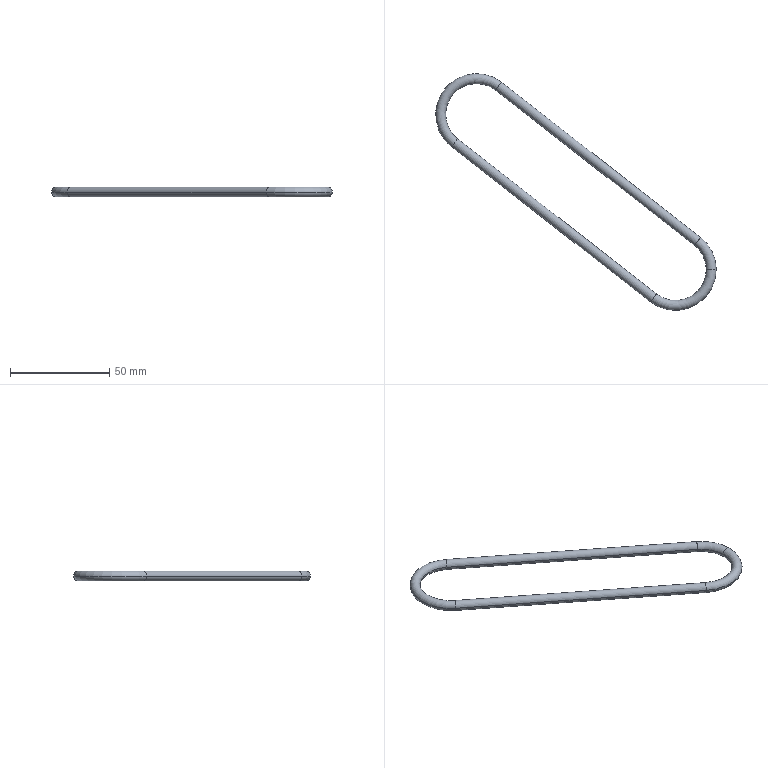Part | STEP file | 10000020599swp000-1 | 1 solid | 10 faces | box 141 x 119 x 5 mm | volume 7201 mm3 | torus 6 | cylinder 4 | commonest cylinder face diameters 5 x4
STEP:
#1=CARTESIAN_POINT('',(-80.467,30.222,-32.));
#2=VERTEX_POINT('',#1);
#3=CARTESIAN_POINT('',(-77.392,34.164,-32.));
#4=VERTEX_POINT('',#3);
#5=CARTESIAN_POINT('',(-78.929,32.193,-32.));
#6=DIRECTION('',(-0.7885,0.615,0.));
#7=DIRECTION('',(-0.615,-0.7885,0.));
#8=AXIS2_PLACEMENT_3D('',#5,#6,#7);
#9=CIRCLE('',#8,2.5);
#10=EDGE_CURVE('',#2,#4,#9,.T.);
#11=ORIENTED_EDGE('',*,*,#10,.T.);
#12=CARTESIAN_POINT('',(-102.608,1.836,-32.));
#13=VERTEX_POINT('',#12);
#14=CARTESIAN_POINT('',(-90.,18.,-32.));
#15=DIRECTION('',(0.,0.,1.));
#16=DIRECTION('',(1.,0.,0.));
#17=AXIS2_PLACEMENT_3D('',#14,#15,#16);
#18=CIRCLE('',#17,20.5);
#19=EDGE_CURVE('',#4,#13,#18,.T.);
#20=ORIENTED_EDGE('',*,*,#19,.T.);
#21=CARTESIAN_POINT('',(-99.533,5.778,-32.));
#22=VERTEX_POINT('',#21);
#23=CARTESIAN_POINT('',(-101.071,3.807,-32.));
#24=DIRECTION('',(0.7885,-0.615,0.));
#25=DIRECTION('',(0.615,0.7885,0.));
#26=AXIS2_PLACEMENT_3D('',#23,#24,#25);
#27=CIRCLE('',#26,2.5);
#28=EDGE_CURVE('',#22,#13,#27,.T.);
#29=ORIENTED_EDGE('',*,*,#28,.F.);
#30=CARTESIAN_POINT('',(-90.,18.,-32.));
#31=DIRECTION('',(0.,0.,1.));
#32=DIRECTION('',(1.,0.,0.));
#33=AXIS2_PLACEMENT_3D('',#30,#31,#32);
#34=CIRCLE('',#33,15.5);
#35=EDGE_CURVE('',#2,#22,#34,.T.);
#36=ORIENTED_EDGE('',*,*,#35,.F.);
#37=EDGE_LOOP('',(#11,#20,#29,#36));
#38=FACE_OUTER_BOUND('',#37,.T.);
#39=CARTESIAN_POINT('',(-90.,18.,-32.));
#40=DIRECTION('',(0.,0.,1.));
#41=DIRECTION('',(1.,0.,0.));
#42=AXIS2_PLACEMENT_3D('',#39,#40,#41);
#43=TOROIDAL_SURFACE('',#42,18.,2.5);
#44=ADVANCED_FACE('',(#38),#43,.T.);
#45=CARTESIAN_POINT('',(30.5,-60.,-32.));
#46=VERTEX_POINT('',#45);
#47=CARTESIAN_POINT('',(25.5,-60.,-32.));
#48=VERTEX_POINT('',#47);
#49=CARTESIAN_POINT('',(28.,-60.,-32.));
#50=DIRECTION('',(0.,-1.,0.));
#51=DIRECTION('',(0.,0.,-1.));
#52=AXIS2_PLACEMENT_3D('',#49,#50,#51);
#53=CIRCLE('',#52,2.5);
#54=EDGE_CURVE('',#46,#48,#53,.T.);
#55=ORIENTED_EDGE('',*,*,#54,.F.);
#56=CARTESIAN_POINT('',(22.608,-43.836,-32.));
#57=VERTEX_POINT('',#56);
#58=CARTESIAN_POINT('',(10.,-60.,-32.));
#59=DIRECTION('',(0.,0.,1.));
#60=DIRECTION('',(1.,0.,0.));
#61=AXIS2_PLACEMENT_3D('',#58,#59,#60);
#62=CIRCLE('',#61,20.5);
#63=EDGE_CURVE('',#46,#57,#62,.T.);
#64=ORIENTED_EDGE('',*,*,#63,.T.);
#65=CARTESIAN_POINT('',(19.533,-47.778,-32.));
#66=VERTEX_POINT('',#65);
#67=CARTESIAN_POINT('',(19.533,-47.778,-32.));
#68=CARTESIAN_POINT('',(19.533,-47.778,-31.673));
#69=CARTESIAN_POINT('',(19.573,-47.727,-31.346));
#70=CARTESIAN_POINT('',(19.727,-47.529,-30.741));
#71=CARTESIAN_POINT('',(19.841,-47.383,-30.464));
#72=CARTESIAN_POINT('',(20.126,-47.018,-30.001));
#73=CARTESIAN_POINT('',(20.296,-46.8,-29.816));
#74=CARTESIAN_POINT('',(20.668,-46.323,-29.565));
#75=CARTESIAN_POINT('',(20.869,-46.065,-29.5));
#76=CARTESIAN_POINT('',(21.272,-45.549,-29.5));
#77=CARTESIAN_POINT('',(21.473,-45.291,-29.565));
#78=CARTESIAN_POINT('',(21.845,-44.814,-29.816));
#79=CARTESIAN_POINT('',(22.015,-44.596,-30.001));
#80=CARTESIAN_POINT('',(22.3,-44.231,-30.464));
#81=CARTESIAN_POINT('',(22.414,-44.085,-30.741));
#82=CARTESIAN_POINT('',(22.568,-43.887,-31.346));
#83=CARTESIAN_POINT('',(22.608,-43.836,-31.673));
#84=CARTESIAN_POINT('',(22.608,-43.836,-32.));
#85=B_SPLINE_CURVE_WITH_KNOTS('',3,(#67,#68,#69,#70,#71,#72,#73,#74,#75,#76,#77,#78,#79,#80,#81,#82,#83,#84),.UNSPECIFIED.,.F.,.F.,(4,2,2,2,2,2,2,2,4),(0.,0.0625,0.125,0.1875,0.25,0.3125,0.375,0.4375,0.5),.UNSPECIFIED.);
#86=EDGE_CURVE('',#66,#57,#85,.T.);
#87=ORIENTED_EDGE('',*,*,#86,.F.);
#88=CARTESIAN_POINT('',(10.,-60.,-32.));
#89=DIRECTION('',(0.,0.,1.));
#90=DIRECTION('',(1.,0.,0.));
#91=AXIS2_PLACEMENT_3D('',#88,#89,#90);
#92=CIRCLE('',#91,15.5);
#93=EDGE_CURVE('',#48,#66,#92,.T.);
#94=ORIENTED_EDGE('',*,*,#93,.F.);
#95=EDGE_LOOP('',(#55,#64,#87,#94));
#96=FACE_OUTER_BOUND('',#95,.T.);
#97=CARTESIAN_POINT('',(10.,-60.,-32.));
#98=DIRECTION('',(0.,0.,1.));
#99=DIRECTION('',(1.,0.,0.));
#100=AXIS2_PLACEMENT_3D('',#97,#98,#99);
#101=TOROIDAL_SURFACE('',#100,18.,2.5);
#102=ADVANCED_FACE('',(#96),#101,.T.);
#103=CARTESIAN_POINT('',(0.467,-72.222,-32.));
#104=VERTEX_POINT('',#103);
#105=CARTESIAN_POINT('',(-2.608,-76.164,-32.));
#106=VERTEX_POINT('',#105);
#107=CARTESIAN_POINT('',(-1.071,-74.193,-32.));
#108=DIRECTION('',(0.7885,-0.615,0.));
#109=DIRECTION('',(0.615,0.7885,0.));
#110=AXIS2_PLACEMENT_3D('',#107,#108,#109);
#111=CIRCLE('',#110,2.5);
#112=EDGE_CURVE('',#104,#106,#111,.T.);
#113=ORIENTED_EDGE('',*,*,#112,.T.);
#114=CARTESIAN_POINT('',(10.,-60.,-32.));
#115=DIRECTION('',(0.,0.,1.));
#116=DIRECTION('',(1.,0.,0.));
#117=AXIS2_PLACEMENT_3D('',#114,#115,#116);
#118=CIRCLE('',#117,20.5);
#119=EDGE_CURVE('',#106,#46,#118,.T.);
#120=ORIENTED_EDGE('',*,*,#119,.T.);
#121=ORIENTED_EDGE('',*,*,#54,.T.);
#122=CARTESIAN_POINT('',(10.,-60.,-32.));
#123=DIRECTION('',(0.,0.,1.));
#124=DIRECTION('',(1.,0.,0.));
#125=AXIS2_PLACEMENT_3D('',#122,#123,#124);
#126=CIRCLE('',#125,15.5);
#127=EDGE_CURVE('',#104,#48,#126,.T.);
#128=ORIENTED_EDGE('',*,*,#127,.F.);
#129=EDGE_LOOP('',(#113,#120,#121,#128));
#130=FACE_OUTER_BOUND('',#129,.T.);
#131=CARTESIAN_POINT('',(10.,-60.,-32.));
#132=DIRECTION('',(0.,0.,1.));
#133=DIRECTION('',(1.,0.,0.));
#134=AXIS2_PLACEMENT_3D('',#131,#132,#133);
#135=TOROIDAL_SURFACE('',#134,18.,2.5);
#136=ADVANCED_FACE('',(#130),#135,.T.);
#137=ORIENTED_EDGE('',*,*,#10,.F.);
#138=CARTESIAN_POINT('',(-80.467,30.222,-32.));
#139=DIRECTION('',(0.7885,-0.615,0.));
#140=VECTOR('',#139,1000.);
#141=LINE('',#138,#140);
#142=EDGE_CURVE('',#2,#66,#141,.T.);
#143=ORIENTED_EDGE('',*,*,#142,.T.);
#144=ORIENTED_EDGE('',*,*,#86,.T.);
#145=CARTESIAN_POINT('',(-77.392,34.164,-32.));
#146=DIRECTION('',(0.7885,-0.615,0.));
#147=VECTOR('',#146,1000.);
#148=LINE('',#145,#147);
#149=EDGE_CURVE('',#4,#57,#148,.T.);
#150=ORIENTED_EDGE('',*,*,#149,.F.);
#151=EDGE_LOOP('',(#137,#143,#144,#150));
#152=FACE_OUTER_BOUND('',#151,.T.);
#153=CARTESIAN_POINT('',(-78.929,32.193,-32.));
#154=DIRECTION('',(0.7885,-0.615,0.));
#155=DIRECTION('',(0.615,0.7885,0.));
#156=AXIS2_PLACEMENT_3D('',#153,#154,#155);
#157=CYLINDRICAL_SURFACE('',#156,2.5);
#158=ADVANCED_FACE('',(#152),#157,.T.);
#159=ORIENTED_EDGE('',*,*,#28,.T.);
#160=CARTESIAN_POINT('',(-102.608,1.836,-32.));
#161=DIRECTION('',(0.7885,-0.615,0.));
#162=VECTOR('',#161,1000.);
#163=LINE('',#160,#162);
#164=EDGE_CURVE('',#13,#106,#163,.T.);
#165=ORIENTED_EDGE('',*,*,#164,.T.);
#166=ORIENTED_EDGE('',*,*,#112,.F.);
#167=CARTESIAN_POINT('',(-99.533,5.778,-32.));
#168=DIRECTION('',(0.7885,-0.615,0.));
#169=VECTOR('',#168,1000.);
#170=LINE('',#167,#169);
#171=EDGE_CURVE('',#22,#104,#170,.T.);
#172=ORIENTED_EDGE('',*,*,#171,.F.);
#173=EDGE_LOOP('',(#159,#165,#166,#172));
#174=FACE_OUTER_BOUND('',#173,.T.);
#175=CARTESIAN_POINT('',(-101.071,3.807,-32.));
#176=DIRECTION('',(0.7885,-0.615,0.));
#177=DIRECTION('',(0.615,0.7885,0.));
#178=AXIS2_PLACEMENT_3D('',#175,#176,#177);
#179=CYLINDRICAL_SURFACE('',#178,2.5);
#180=ADVANCED_FACE('',(#174),#179,.T.);
#181=ORIENTED_EDGE('',*,*,#119,.F.);
#182=CARTESIAN_POINT('',(-1.071,-74.193,-32.));
#183=DIRECTION('',(0.7885,-0.615,0.));
#184=DIRECTION('',(0.615,0.7885,0.));
#185=AXIS2_PLACEMENT_3D('',#182,#183,#184);
#186=CIRCLE('',#185,2.5);
#187=EDGE_CURVE('',#106,#104,#186,.T.);
#188=ORIENTED_EDGE('',*,*,#187,.T.);
#189=ORIENTED_EDGE('',*,*,#127,.T.);
#190=CARTESIAN_POINT('',(28.,-60.,-32.));
#191=DIRECTION('',(0.,-1.,0.));
#192=DIRECTION('',(0.,0.,-1.));
#193=AXIS2_PLACEMENT_3D('',#190,#191,#192);
#194=CIRCLE('',#193,2.5);
#195=EDGE_CURVE('',#48,#46,#194,.T.);
#196=ORIENTED_EDGE('',*,*,#195,.T.);
#197=EDGE_LOOP('',(#181,#188,#189,#196));
#198=FACE_OUTER_BOUND('',#197,.T.);
#199=CARTESIAN_POINT('',(10.,-60.,-32.));
#200=DIRECTION('',(0.,0.,1.));
#201=DIRECTION('',(1.,0.,0.));
#202=AXIS2_PLACEMENT_3D('',#199,#200,#201);
#203=TOROIDAL_SURFACE('',#202,18.,2.5);
#204=ADVANCED_FACE('',(#198),#203,.T.);
#205=ORIENTED_EDGE('',*,*,#63,.F.);
#206=ORIENTED_EDGE('',*,*,#195,.F.);
#207=ORIENTED_EDGE('',*,*,#93,.T.);
#208=CARTESIAN_POINT('',(22.608,-43.836,-32.));
#209=CARTESIAN_POINT('',(22.608,-43.836,-32.327));
#210=CARTESIAN_POINT('',(22.568,-43.887,-32.654));
#211=CARTESIAN_POINT('',(22.414,-44.085,-33.259));
#212=CARTESIAN_POINT('',(22.3,-44.231,-33.536));
#213=CARTESIAN_POINT('',(22.015,-44.596,-33.999));
#214=CARTESIAN_POINT('',(21.845,-44.814,-34.184));
#215=CARTESIAN_POINT('',(21.473,-45.291,-34.435));
#216=CARTESIAN_POINT('',(21.272,-45.549,-34.5));
#217=CARTESIAN_POINT('',(20.869,-46.065,-34.5));
#218=CARTESIAN_POINT('',(20.668,-46.323,-34.435));
#219=CARTESIAN_POINT('',(20.296,-46.8,-34.184));
#220=CARTESIAN_POINT('',(20.126,-47.018,-33.999));
#221=CARTESIAN_POINT('',(19.841,-47.383,-33.536));
#222=CARTESIAN_POINT('',(19.727,-47.529,-33.259));
#223=CARTESIAN_POINT('',(19.573,-47.727,-32.654));
#224=CARTESIAN_POINT('',(19.533,-47.778,-32.327));
#225=CARTESIAN_POINT('',(19.533,-47.778,-32.));
#226=B_SPLINE_CURVE_WITH_KNOTS('',3,(#208,#209,#210,#211,#212,#213,#214,#215,#216,#217,#218,#219,#220,#221,#222,#223,#224,#225),.UNSPECIFIED.,.F.,.F.,(4,2,2,2,2,2,2,2,4),(0.5,0.5625,0.625,0.6875,0.75,0.8125,0.875,0.9375,1.),.UNSPECIFIED.);
#227=EDGE_CURVE('',#57,#66,#226,.T.);
#228=ORIENTED_EDGE('',*,*,#227,.F.);
#229=EDGE_LOOP('',(#205,#206,#207,#228));
#230=FACE_OUTER_BOUND('',#229,.T.);
#231=CARTESIAN_POINT('',(10.,-60.,-32.));
#232=DIRECTION('',(0.,0.,1.));
#233=DIRECTION('',(1.,0.,0.));
#234=AXIS2_PLACEMENT_3D('',#231,#232,#233);
#235=TOROIDAL_SURFACE('',#234,18.,2.5);
#236=ADVANCED_FACE('',(#230),#235,.T.);
#237=ORIENTED_EDGE('',*,*,#164,.F.);
#238=CARTESIAN_POINT('',(-101.071,3.807,-32.));
#239=DIRECTION('',(0.7885,-0.615,0.));
#240=DIRECTION('',(0.615,0.7885,0.));
#241=AXIS2_PLACEMENT_3D('',#238,#239,#240);
#242=CIRCLE('',#241,2.5);
#243=EDGE_CURVE('',#13,#22,#242,.T.);
#244=ORIENTED_EDGE('',*,*,#243,.T.);
#245=ORIENTED_EDGE('',*,*,#171,.T.);
#246=ORIENTED_EDGE('',*,*,#187,.F.);
#247=EDGE_LOOP('',(#237,#244,#245,#246));
#248=FACE_OUTER_BOUND('',#247,.T.);
#249=CARTESIAN_POINT('',(-101.071,3.807,-32.));
#250=DIRECTION('',(0.7885,-0.615,0.));
#251=DIRECTION('',(0.615,0.7885,0.));
#252=AXIS2_PLACEMENT_3D('',#249,#250,#251);
#253=CYLINDRICAL_SURFACE('',#252,2.5);
#254=ADVANCED_FACE('',(#248),#253,.T.);
#255=ORIENTED_EDGE('',*,*,#19,.F.);
#256=CARTESIAN_POINT('',(-78.929,32.193,-32.));
#257=DIRECTION('',(-0.7885,0.615,0.));
#258=DIRECTION('',(-0.615,-0.7885,0.));
#259=AXIS2_PLACEMENT_3D('',#256,#257,#258);
#260=CIRCLE('',#259,2.5);
#261=EDGE_CURVE('',#4,#2,#260,.T.);
#262=ORIENTED_EDGE('',*,*,#261,.T.);
#263=ORIENTED_EDGE('',*,*,#35,.T.);
#264=ORIENTED_EDGE('',*,*,#243,.F.);
#265=EDGE_LOOP('',(#255,#262,#263,#264));
#266=FACE_OUTER_BOUND('',#265,.T.);
#267=CARTESIAN_POINT('',(-90.,18.,-32.));
#268=DIRECTION('',(0.,0.,1.));
#269=DIRECTION('',(1.,0.,0.));
#270=AXIS2_PLACEMENT_3D('',#267,#268,#269);
#271=TOROIDAL_SURFACE('',#270,18.,2.5);
#272=ADVANCED_FACE('',(#266),#271,.T.);
#273=ORIENTED_EDGE('',*,*,#142,.F.);
#274=ORIENTED_EDGE('',*,*,#261,.F.);
#275=ORIENTED_EDGE('',*,*,#149,.T.);
#276=ORIENTED_EDGE('',*,*,#227,.T.);
#277=EDGE_LOOP('',(#273,#274,#275,#276));
#278=FACE_OUTER_BOUND('',#277,.T.);
#279=CARTESIAN_POINT('',(-78.929,32.193,-32.));
#280=DIRECTION('',(0.7885,-0.615,0.));
#281=DIRECTION('',(0.615,0.7885,0.));
#282=AXIS2_PLACEMENT_3D('',#279,#280,#281);
#283=CYLINDRICAL_SURFACE('',#282,2.5);
#284=ADVANCED_FACE('',(#278),#283,.T.);
#285=CLOSED_SHELL('',(#44,#102,#136,#158,#180,#204,#236,#254,#272,#284));
#286=MANIFOLD_SOLID_BREP('',#285);
#287=CARTESIAN_POINT('',(0.,0.,0.));
#288=DIRECTION('',(0.,0.,1.));
#289=DIRECTION('',(1.,0.,0.));
#290=AXIS2_PLACEMENT_3D('',#287,#288,#289);
#291=(LENGTH_UNIT()NAMED_UNIT(*)SI_UNIT(.MILLI.,.METRE.));
#292=UNCERTAINTY_MEASURE_WITH_UNIT(LENGTH_MEASURE(0.00001),#291,'','');
#293=(NAMED_UNIT(*)PLANE_ANGLE_UNIT()SI_UNIT($,.RADIAN.));
#294=(NAMED_UNIT(*)SI_UNIT($,.STERADIAN.)SOLID_ANGLE_UNIT());
#295=(GEOMETRIC_REPRESENTATION_CONTEXT(3)GLOBAL_UNCERTAINTY_ASSIGNED_CONTEXT((#292))GLOBAL_UNIT_ASSIGNED_CONTEXT((#291,#293,#294))REPRESENTATION_CONTEXT('',''));
#296=ADVANCED_BREP_SHAPE_REPRESENTATION('',(#286,#290),#295);